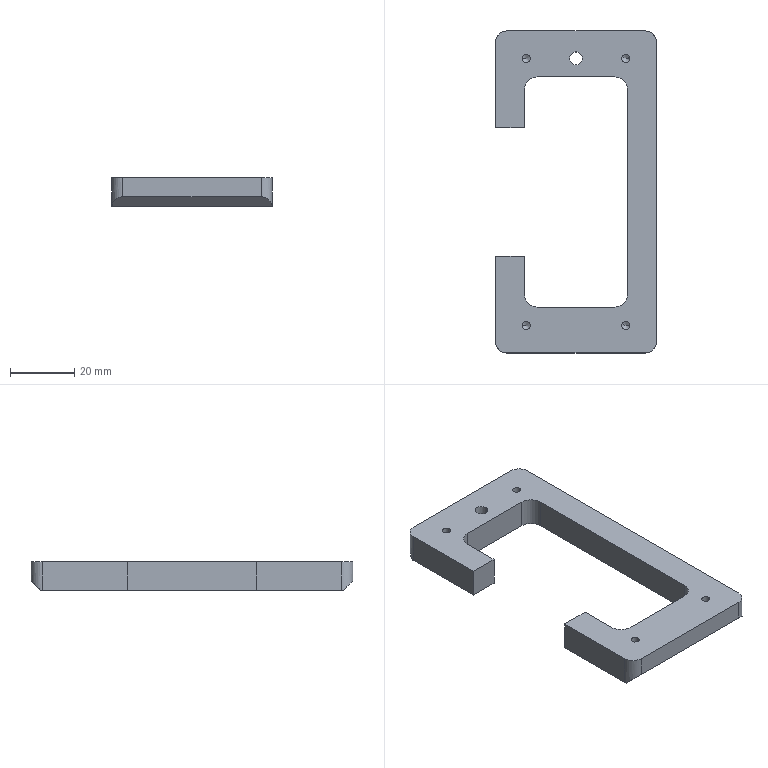Part | STEP file | X77-02213 | 1 solid | 42 faces | box 50 x 100 x 9 mm | volume 20503 mm3 | cylinder 18 | plane 16 | cone 8 | commonest cylinder face diameters 2.5 x8 7.116 x4 8 x4 4 x2
STEP:
#1=CARTESIAN_POINT('',(-2.,41.5,0.));
#2=VERTEX_POINT('',#1);
#3=CARTESIAN_POINT('',(2.,41.5,0.));
#4=VERTEX_POINT('',#3);
#5=CARTESIAN_POINT('',(-0.000000005,41.5,0.));
#6=DIRECTION('',(0.,0.,-1.));
#7=DIRECTION('',(1.,0.,0.));
#8=AXIS2_PLACEMENT_3D('',#5,#6,#7);
#9=CIRCLE('',#8,2.);
#10=EDGE_CURVE('',#2,#4,#9,.T.);
#11=ORIENTED_EDGE('',*,*,#10,.T.);
#12=CARTESIAN_POINT('',(2.,41.5,9.));
#13=VERTEX_POINT('',#12);
#14=CARTESIAN_POINT('',(2.,41.5,-1.));
#15=DIRECTION('',(0.,0.,1.));
#16=VECTOR('',#15,1000.);
#17=LINE('',#14,#16);
#18=EDGE_CURVE('',#4,#13,#17,.T.);
#19=ORIENTED_EDGE('',*,*,#18,.T.);
#20=CARTESIAN_POINT('',(-2.,41.5,9.));
#21=VERTEX_POINT('',#20);
#22=CARTESIAN_POINT('',(-0.000000005,41.5,9.));
#23=DIRECTION('',(0.,0.,1.));
#24=DIRECTION('',(-1.,0.,0.));
#25=AXIS2_PLACEMENT_3D('',#22,#23,#24);
#26=CIRCLE('',#25,2.);
#27=EDGE_CURVE('',#13,#21,#26,.T.);
#28=ORIENTED_EDGE('',*,*,#27,.T.);
#29=CARTESIAN_POINT('',(-2.,41.5,-1.));
#30=DIRECTION('',(0.,0.,1.));
#31=VECTOR('',#30,1000.);
#32=LINE('',#29,#31);
#33=EDGE_CURVE('',#2,#21,#32,.T.);
#34=ORIENTED_EDGE('',*,*,#33,.F.);
#35=EDGE_LOOP('',(#11,#19,#28,#34));
#36=FACE_OUTER_BOUND('',#35,.T.);
#37=CARTESIAN_POINT('',(-0.000000005,41.5,-1.));
#38=DIRECTION('',(0.,0.,1.));
#39=DIRECTION('',(-1.,0.,0.));
#40=AXIS2_PLACEMENT_3D('',#37,#38,#39);
#41=CYLINDRICAL_SURFACE('',#40,2.);
#42=ADVANCED_FACE('',(#36),#41,.F.);
#43=CARTESIAN_POINT('',(16.75,41.5,1.5));
#44=VERTEX_POINT('',#43);
#45=CARTESIAN_POINT('',(14.25,41.5,1.5));
#46=VERTEX_POINT('',#45);
#47=CARTESIAN_POINT('',(15.5,41.5,1.5));
#48=DIRECTION('',(0.,0.,1.));
#49=DIRECTION('',(-1.,0.,0.));
#50=AXIS2_PLACEMENT_3D('',#47,#48,#49);
#51=CIRCLE('',#50,1.25);
#52=EDGE_CURVE('',#44,#46,#51,.T.);
#53=ORIENTED_EDGE('',*,*,#52,.F.);
#54=CARTESIAN_POINT('',(16.75,41.5,9.));
#55=VERTEX_POINT('',#54);
#56=CARTESIAN_POINT('',(16.75,41.5,9.));
#57=DIRECTION('',(0.,0.,1.));
#58=VECTOR('',#57,1000.);
#59=LINE('',#56,#58);
#60=EDGE_CURVE('',#44,#55,#59,.T.);
#61=ORIENTED_EDGE('',*,*,#60,.T.);
#62=CARTESIAN_POINT('',(14.25,41.5,9.));
#63=VERTEX_POINT('',#62);
#64=CARTESIAN_POINT('',(15.5,41.5,9.));
#65=DIRECTION('',(0.,0.,1.));
#66=DIRECTION('',(-1.,0.,0.));
#67=AXIS2_PLACEMENT_3D('',#64,#65,#66);
#68=CIRCLE('',#67,1.25);
#69=EDGE_CURVE('',#55,#63,#68,.T.);
#70=ORIENTED_EDGE('',*,*,#69,.T.);
#71=CARTESIAN_POINT('',(14.25,41.5,9.));
#72=DIRECTION('',(0.,0.,1.));
#73=VECTOR('',#72,1000.);
#74=LINE('',#71,#73);
#75=EDGE_CURVE('',#46,#63,#74,.T.);
#76=ORIENTED_EDGE('',*,*,#75,.F.);
#77=EDGE_LOOP('',(#53,#61,#70,#76));
#78=FACE_OUTER_BOUND('',#77,.T.);
#79=CARTESIAN_POINT('',(15.5,41.5,9.));
#80=DIRECTION('',(0.,0.,1.));
#81=DIRECTION('',(-1.,0.,0.));
#82=AXIS2_PLACEMENT_3D('',#79,#80,#81);
#83=CYLINDRICAL_SURFACE('',#82,1.25);
#84=ADVANCED_FACE('',(#78),#83,.F.);
#85=CARTESIAN_POINT('',(15.5,41.5,0.7489));
#86=VERTEX_POINT('',#85);
#87=CARTESIAN_POINT('',(14.25,41.5,1.5));
#88=DIRECTION('',(-0.8572,0.,0.515));
#89=VECTOR('',#88,1000.);
#90=LINE('',#87,#89);
#91=EDGE_CURVE('',#86,#46,#90,.T.);
#92=ORIENTED_EDGE('',*,*,#91,.F.);
#93=CARTESIAN_POINT('',(16.75,41.5,1.5));
#94=DIRECTION('',(0.8572,0.,0.515));
#95=VECTOR('',#94,1000.);
#96=LINE('',#93,#95);
#97=EDGE_CURVE('',#86,#44,#96,.T.);
#98=ORIENTED_EDGE('',*,*,#97,.T.);
#99=ORIENTED_EDGE('',*,*,#52,.T.);
#100=EDGE_LOOP('',(#92,#98,#99));
#101=FACE_OUTER_BOUND('',#100,.T.);
#102=CARTESIAN_POINT('',(15.5,41.5,1.5));
#103=DIRECTION('',(0.,0.,1.));
#104=DIRECTION('',(-1.,0.,0.));
#105=AXIS2_PLACEMENT_3D('',#102,#103,#104);
#106=CONICAL_SURFACE('',#105,1.25,1.03);
#107=ADVANCED_FACE('',(#101),#106,.F.);
#108=CARTESIAN_POINT('',(-14.25,41.5,1.5));
#109=VERTEX_POINT('',#108);
#110=CARTESIAN_POINT('',(-16.75,41.5,1.5));
#111=VERTEX_POINT('',#110);
#112=CARTESIAN_POINT('',(-15.5,41.5,1.5));
#113=DIRECTION('',(0.,0.,1.));
#114=DIRECTION('',(-1.,0.,0.));
#115=AXIS2_PLACEMENT_3D('',#112,#113,#114);
#116=CIRCLE('',#115,1.25);
#117=EDGE_CURVE('',#109,#111,#116,.T.);
#118=ORIENTED_EDGE('',*,*,#117,.F.);
#119=CARTESIAN_POINT('',(-14.25,41.5,9.));
#120=VERTEX_POINT('',#119);
#121=CARTESIAN_POINT('',(-14.25,41.5,9.));
#122=DIRECTION('',(0.,0.,1.));
#123=VECTOR('',#122,1000.);
#124=LINE('',#121,#123);
#125=EDGE_CURVE('',#109,#120,#124,.T.);
#126=ORIENTED_EDGE('',*,*,#125,.T.);
#127=CARTESIAN_POINT('',(-16.75,41.5,9.));
#128=VERTEX_POINT('',#127);
#129=CARTESIAN_POINT('',(-15.5,41.5,9.));
#130=DIRECTION('',(0.,0.,1.));
#131=DIRECTION('',(-1.,0.,0.));
#132=AXIS2_PLACEMENT_3D('',#129,#130,#131);
#133=CIRCLE('',#132,1.25);
#134=EDGE_CURVE('',#120,#128,#133,.T.);
#135=ORIENTED_EDGE('',*,*,#134,.T.);
#136=CARTESIAN_POINT('',(-16.75,41.5,9.));
#137=DIRECTION('',(0.,0.,1.));
#138=VECTOR('',#137,1000.);
#139=LINE('',#136,#138);
#140=EDGE_CURVE('',#111,#128,#139,.T.);
#141=ORIENTED_EDGE('',*,*,#140,.F.);
#142=EDGE_LOOP('',(#118,#126,#135,#141));
#143=FACE_OUTER_BOUND('',#142,.T.);
#144=CARTESIAN_POINT('',(-15.5,41.5,9.));
#145=DIRECTION('',(0.,0.,1.));
#146=DIRECTION('',(-1.,0.,0.));
#147=AXIS2_PLACEMENT_3D('',#144,#145,#146);
#148=CYLINDRICAL_SURFACE('',#147,1.25);
#149=ADVANCED_FACE('',(#143),#148,.F.);
#150=CARTESIAN_POINT('',(-15.5,41.5,0.7489));
#151=VERTEX_POINT('',#150);
#152=CARTESIAN_POINT('',(-16.75,41.5,1.5));
#153=DIRECTION('',(-0.8572,0.,0.515));
#154=VECTOR('',#153,1000.);
#155=LINE('',#152,#154);
#156=EDGE_CURVE('',#151,#111,#155,.T.);
#157=ORIENTED_EDGE('',*,*,#156,.F.);
#158=CARTESIAN_POINT('',(-14.25,41.5,1.5));
#159=DIRECTION('',(0.8572,0.,0.515));
#160=VECTOR('',#159,1000.);
#161=LINE('',#158,#160);
#162=EDGE_CURVE('',#151,#109,#161,.T.);
#163=ORIENTED_EDGE('',*,*,#162,.T.);
#164=ORIENTED_EDGE('',*,*,#117,.T.);
#165=EDGE_LOOP('',(#157,#163,#164));
#166=FACE_OUTER_BOUND('',#165,.T.);
#167=CARTESIAN_POINT('',(-15.5,41.5,1.5));
#168=DIRECTION('',(0.,0.,1.));
#169=DIRECTION('',(-1.,0.,0.));
#170=AXIS2_PLACEMENT_3D('',#167,#168,#169);
#171=CONICAL_SURFACE('',#170,1.25,1.03);
#172=ADVANCED_FACE('',(#166),#171,.F.);
#173=CARTESIAN_POINT('',(-14.25,-41.5,1.5));
#174=VERTEX_POINT('',#173);
#175=CARTESIAN_POINT('',(-16.75,-41.5,1.5));
#176=VERTEX_POINT('',#175);
#177=CARTESIAN_POINT('',(-15.5,-41.5,1.5));
#178=DIRECTION('',(0.,0.,1.));
#179=DIRECTION('',(-1.,0.,0.));
#180=AXIS2_PLACEMENT_3D('',#177,#178,#179);
#181=CIRCLE('',#180,1.25);
#182=EDGE_CURVE('',#174,#176,#181,.T.);
#183=ORIENTED_EDGE('',*,*,#182,.F.);
#184=CARTESIAN_POINT('',(-14.25,-41.5,9.));
#185=VERTEX_POINT('',#184);
#186=CARTESIAN_POINT('',(-14.25,-41.5,9.));
#187=DIRECTION('',(0.,0.,1.));
#188=VECTOR('',#187,1000.);
#189=LINE('',#186,#188);
#190=EDGE_CURVE('',#174,#185,#189,.T.);
#191=ORIENTED_EDGE('',*,*,#190,.T.);
#192=CARTESIAN_POINT('',(-16.75,-41.5,9.));
#193=VERTEX_POINT('',#192);
#194=CARTESIAN_POINT('',(-15.5,-41.5,9.));
#195=DIRECTION('',(0.,0.,1.));
#196=DIRECTION('',(-1.,0.,0.));
#197=AXIS2_PLACEMENT_3D('',#194,#195,#196);
#198=CIRCLE('',#197,1.25);
#199=EDGE_CURVE('',#185,#193,#198,.T.);
#200=ORIENTED_EDGE('',*,*,#199,.T.);
#201=CARTESIAN_POINT('',(-16.75,-41.5,9.));
#202=DIRECTION('',(0.,0.,1.));
#203=VECTOR('',#202,1000.);
#204=LINE('',#201,#203);
#205=EDGE_CURVE('',#176,#193,#204,.T.);
#206=ORIENTED_EDGE('',*,*,#205,.F.);
#207=EDGE_LOOP('',(#183,#191,#200,#206));
#208=FACE_OUTER_BOUND('',#207,.T.);
#209=CARTESIAN_POINT('',(-15.5,-41.5,9.));
#210=DIRECTION('',(0.,0.,1.));
#211=DIRECTION('',(-1.,0.,0.));
#212=AXIS2_PLACEMENT_3D('',#209,#210,#211);
#213=CYLINDRICAL_SURFACE('',#212,1.25);
#214=ADVANCED_FACE('',(#208),#213,.F.);
#215=CARTESIAN_POINT('',(-15.5,-41.5,0.7489));
#216=VERTEX_POINT('',#215);
#217=CARTESIAN_POINT('',(-16.75,-41.5,1.5));
#218=DIRECTION('',(-0.8572,0.,0.515));
#219=VECTOR('',#218,1000.);
#220=LINE('',#217,#219);
#221=EDGE_CURVE('',#216,#176,#220,.T.);
#222=ORIENTED_EDGE('',*,*,#221,.F.);
#223=CARTESIAN_POINT('',(-14.25,-41.5,1.5));
#224=DIRECTION('',(0.8572,0.,0.515));
#225=VECTOR('',#224,1000.);
#226=LINE('',#223,#225);
#227=EDGE_CURVE('',#216,#174,#226,.T.);
#228=ORIENTED_EDGE('',*,*,#227,.T.);
#229=ORIENTED_EDGE('',*,*,#182,.T.);
#230=EDGE_LOOP('',(#222,#228,#229));
#231=FACE_OUTER_BOUND('',#230,.T.);
#232=CARTESIAN_POINT('',(-15.5,-41.5,1.5));
#233=DIRECTION('',(0.,0.,1.));
#234=DIRECTION('',(-1.,0.,0.));
#235=AXIS2_PLACEMENT_3D('',#232,#233,#234);
#236=CONICAL_SURFACE('',#235,1.25,1.03);
#237=ADVANCED_FACE('',(#231),#236,.F.);
#238=CARTESIAN_POINT('',(16.75,-41.5,1.5));
#239=VERTEX_POINT('',#238);
#240=CARTESIAN_POINT('',(14.25,-41.5,1.5));
#241=VERTEX_POINT('',#240);
#242=CARTESIAN_POINT('',(15.5,-41.5,1.5));
#243=DIRECTION('',(0.,0.,1.));
#244=DIRECTION('',(-1.,0.,0.));
#245=AXIS2_PLACEMENT_3D('',#242,#243,#244);
#246=CIRCLE('',#245,1.25);
#247=EDGE_CURVE('',#239,#241,#246,.T.);
#248=ORIENTED_EDGE('',*,*,#247,.F.);
#249=CARTESIAN_POINT('',(16.75,-41.5,9.));
#250=VERTEX_POINT('',#249);
#251=CARTESIAN_POINT('',(16.75,-41.5,9.));
#252=DIRECTION('',(0.,0.,1.));
#253=VECTOR('',#252,1000.);
#254=LINE('',#251,#253);
#255=EDGE_CURVE('',#239,#250,#254,.T.);
#256=ORIENTED_EDGE('',*,*,#255,.T.);
#257=CARTESIAN_POINT('',(14.25,-41.5,9.));
#258=VERTEX_POINT('',#257);
#259=CARTESIAN_POINT('',(15.5,-41.5,9.));
#260=DIRECTION('',(0.,0.,1.));
#261=DIRECTION('',(-1.,0.,0.));
#262=AXIS2_PLACEMENT_3D('',#259,#260,#261);
#263=CIRCLE('',#262,1.25);
#264=EDGE_CURVE('',#250,#258,#263,.T.);
#265=ORIENTED_EDGE('',*,*,#264,.T.);
#266=CARTESIAN_POINT('',(14.25,-41.5,9.));
#267=DIRECTION('',(0.,0.,1.));
#268=VECTOR('',#267,1000.);
#269=LINE('',#266,#268);
#270=EDGE_CURVE('',#241,#258,#269,.T.);
#271=ORIENTED_EDGE('',*,*,#270,.F.);
#272=EDGE_LOOP('',(#248,#256,#265,#271));
#273=FACE_OUTER_BOUND('',#272,.T.);
#274=CARTESIAN_POINT('',(15.5,-41.5,9.));
#275=DIRECTION('',(0.,0.,1.));
#276=DIRECTION('',(-1.,0.,0.));
#277=AXIS2_PLACEMENT_3D('',#274,#275,#276);
#278=CYLINDRICAL_SURFACE('',#277,1.25);
#279=ADVANCED_FACE('',(#273),#278,.F.);
#280=CARTESIAN_POINT('',(15.5,-41.5,0.7489));
#281=VERTEX_POINT('',#280);
#282=CARTESIAN_POINT('',(14.25,-41.5,1.5));
#283=DIRECTION('',(-0.8572,0.,0.515));
#284=VECTOR('',#283,1000.);
#285=LINE('',#282,#284);
#286=EDGE_CURVE('',#281,#241,#285,.T.);
#287=ORIENTED_EDGE('',*,*,#286,.F.);
#288=CARTESIAN_POINT('',(16.75,-41.5,1.5));
#289=DIRECTION('',(0.8572,0.,0.515));
#290=VECTOR('',#289,1000.);
#291=LINE('',#288,#290);
#292=EDGE_CURVE('',#281,#239,#291,.T.);
#293=ORIENTED_EDGE('',*,*,#292,.T.);
#294=ORIENTED_EDGE('',*,*,#247,.T.);
#295=EDGE_LOOP('',(#287,#293,#294));
#296=FACE_OUTER_BOUND('',#295,.T.);
#297=CARTESIAN_POINT('',(15.5,-41.5,1.5));
#298=DIRECTION('',(0.,0.,1.));
#299=DIRECTION('',(-1.,0.,0.));
#300=AXIS2_PLACEMENT_3D('',#297,#298,#299);
#301=CONICAL_SURFACE('',#300,1.25,1.03);
#302=ADVANCED_FACE('',(#296),#301,.F.);
#303=CARTESIAN_POINT('',(-25.,-20.,9.));
#304=VERTEX_POINT('',#303);
#305=CARTESIAN_POINT('',(-25.,-46.442,9.));
#306=VERTEX_POINT('',#305);
#307=CARTESIAN_POINT('',(-25.,50.,9.));
#308=DIRECTION('',(0.,-1.,0.));
#309=VECTOR('',#308,1000.);
#310=LINE('',#307,#309);
#311=EDGE_CURVE('',#304,#306,#310,.T.);
#312=ORIENTED_EDGE('',*,*,#311,.F.);
#313=CARTESIAN_POINT('',(-25.,-20.,0.));
#314=VERTEX_POINT('',#313);
#315=CARTESIAN_POINT('',(-25.,-20.,-11.867));
#316=DIRECTION('',(0.,0.,1.));
#317=VECTOR('',#316,1000.);
#318=LINE('',#315,#317);
#319=EDGE_CURVE('',#314,#304,#318,.T.);
#320=ORIENTED_EDGE('',*,*,#319,.F.);
#321=CARTESIAN_POINT('',(-25.,-46.442,0.));
#322=VERTEX_POINT('',#321);
#323=CARTESIAN_POINT('',(-25.,46.442,0.));
#324=DIRECTION('',(0.,-1.,0.));
#325=VECTOR('',#324,1000.);
#326=LINE('',#323,#325);
#327=EDGE_CURVE('',#314,#322,#326,.T.);
#328=ORIENTED_EDGE('',*,*,#327,.T.);
#329=CARTESIAN_POINT('',(-25.,-46.442,10.));
#330=DIRECTION('',(0.,0.,-1.));
#331=VECTOR('',#330,1000.);
#332=LINE('',#329,#331);
#333=EDGE_CURVE('',#306,#322,#332,.T.);
#334=ORIENTED_EDGE('',*,*,#333,.F.);
#335=EDGE_LOOP('',(#312,#320,#328,#334));
#336=FACE_OUTER_BOUND('',#335,.T.);
#337=CARTESIAN_POINT('',(-25.,46.442,10.));
#338=DIRECTION('',(1.,0.,0.));
#339=DIRECTION('',(0.,0.,-1.));
#340=AXIS2_PLACEMENT_3D('',#337,#338,#339);
#341=PLANE('',#340);
#342=ADVANCED_FACE('',(#336),#341,.F.);
#343=CARTESIAN_POINT('',(-16.,-20.,9.));
#344=VERTEX_POINT('',#343);
#345=CARTESIAN_POINT('',(-16.,-20.,0.));
#346=VERTEX_POINT('',#345);
#347=CARTESIAN_POINT('',(-16.,-20.,10.));
#348=DIRECTION('',(0.,0.,-1.));
#349=VECTOR('',#348,1000.);
#350=LINE('',#347,#349);
#351=EDGE_CURVE('',#344,#346,#350,.T.);
#352=ORIENTED_EDGE('',*,*,#351,.F.);
#353=CARTESIAN_POINT('',(-16.,-31.75,9.));
#354=VERTEX_POINT('',#353);
#355=CARTESIAN_POINT('',(-16.,-31.75,9.));
#356=DIRECTION('',(0.,1.,0.));
#357=VECTOR('',#356,1000.);
#358=LINE('',#355,#357);
#359=EDGE_CURVE('',#354,#344,#358,.T.);
#360=ORIENTED_EDGE('',*,*,#359,.F.);
#361=CARTESIAN_POINT('',(-16.,-31.75,0.));
#362=VERTEX_POINT('',#361);
#363=CARTESIAN_POINT('',(-16.,-31.75,10.));
#364=DIRECTION('',(0.,0.,-1.));
#365=VECTOR('',#364,1000.);
#366=LINE('',#363,#365);
#367=EDGE_CURVE('',#354,#362,#366,.T.);
#368=ORIENTED_EDGE('',*,*,#367,.T.);
#369=CARTESIAN_POINT('',(-16.,-31.75,0.));
#370=DIRECTION('',(0.,-1.,0.));
#371=VECTOR('',#370,1000.);
#372=LINE('',#369,#371);
#373=EDGE_CURVE('',#346,#362,#372,.T.);
#374=ORIENTED_EDGE('',*,*,#373,.F.);
#375=EDGE_LOOP('',(#352,#360,#368,#374));
#376=FACE_OUTER_BOUND('',#375,.T.);
#377=CARTESIAN_POINT('',(-16.,-31.75,10.));
#378=DIRECTION('',(1.,0.,0.));
#379=DIRECTION('',(0.,1.,0.));
#380=AXIS2_PLACEMENT_3D('',#377,#378,#379);
#381=PLANE('',#380);
#382=ADVANCED_FACE('',(#376),#381,.T.);
#383=CARTESIAN_POINT('',(21.442,-20.,0.));
#384=DIRECTION('',(-1.,0.,0.));
#385=VECTOR('',#384,1000.);
#386=LINE('',#383,#385);
#387=EDGE_CURVE('',#346,#314,#386,.T.);
#388=ORIENTED_EDGE('',*,*,#387,.F.);
#389=ORIENTED_EDGE('',*,*,#373,.T.);
#390=CARTESIAN_POINT('',(-12.,-35.75,0.));
#391=VERTEX_POINT('',#390);
#392=CARTESIAN_POINT('',(-12.,-31.75,0.));
#393=DIRECTION('',(0.,0.,1.));
#394=DIRECTION('',(-1.,0.,0.));
#395=AXIS2_PLACEMENT_3D('',#392,#393,#394);
#396=CIRCLE('',#395,4.);
#397=EDGE_CURVE('',#362,#391,#396,.T.);
#398=ORIENTED_EDGE('',*,*,#397,.T.);
#399=CARTESIAN_POINT('',(12.,-35.75,0.));
#400=VERTEX_POINT('',#399);
#401=CARTESIAN_POINT('',(-12.,-35.75,0.));
#402=DIRECTION('',(1.,0.,0.));
#403=VECTOR('',#402,1000.);
#404=LINE('',#401,#403);
#405=EDGE_CURVE('',#391,#400,#404,.T.);
#406=ORIENTED_EDGE('',*,*,#405,.T.);
#407=CARTESIAN_POINT('',(16.,-31.75,0.));
#408=VERTEX_POINT('',#407);
#409=CARTESIAN_POINT('',(12.,-31.75,0.));
#410=DIRECTION('',(0.,0.,1.));
#411=DIRECTION('',(-1.,0.,0.));
#412=AXIS2_PLACEMENT_3D('',#409,#410,#411);
#413=CIRCLE('',#412,4.);
#414=EDGE_CURVE('',#400,#408,#413,.T.);
#415=ORIENTED_EDGE('',*,*,#414,.T.);
#416=CARTESIAN_POINT('',(16.,31.75,0.));
#417=VERTEX_POINT('',#416);
#418=CARTESIAN_POINT('',(16.,-31.75,0.));
#419=DIRECTION('',(0.,1.,0.));
#420=VECTOR('',#419,1000.);
#421=LINE('',#418,#420);
#422=EDGE_CURVE('',#408,#417,#421,.T.);
#423=ORIENTED_EDGE('',*,*,#422,.T.);
#424=CARTESIAN_POINT('',(12.,35.75,0.));
#425=VERTEX_POINT('',#424);
#426=CARTESIAN_POINT('',(12.,31.75,0.));
#427=DIRECTION('',(0.,0.,1.));
#428=DIRECTION('',(1.,0.,0.));
#429=AXIS2_PLACEMENT_3D('',#426,#427,#428);
#430=CIRCLE('',#429,4.);
#431=EDGE_CURVE('',#417,#425,#430,.T.);
#432=ORIENTED_EDGE('',*,*,#431,.T.);
#433=CARTESIAN_POINT('',(-12.,35.75,0.));
#434=VERTEX_POINT('',#433);
#435=CARTESIAN_POINT('',(-12.,35.75,0.));
#436=DIRECTION('',(-1.,0.,0.));
#437=VECTOR('',#436,1000.);
#438=LINE('',#435,#437);
#439=EDGE_CURVE('',#425,#434,#438,.T.);
#440=ORIENTED_EDGE('',*,*,#439,.T.);
#441=CARTESIAN_POINT('',(-16.,31.75,0.));
#442=VERTEX_POINT('',#441);
#443=CARTESIAN_POINT('',(-12.,31.75,0.));
#444=DIRECTION('',(0.,0.,1.));
#445=DIRECTION('',(1.,0.,0.));
#446=AXIS2_PLACEMENT_3D('',#443,#444,#445);
#447=CIRCLE('',#446,4.);
#448=EDGE_CURVE('',#434,#442,#447,.T.);
#449=ORIENTED_EDGE('',*,*,#448,.T.);
#450=CARTESIAN_POINT('',(-16.,20.,0.));
#451=VERTEX_POINT('',#450);
#452=CARTESIAN_POINT('',(-16.,-31.75,0.));
#453=DIRECTION('',(0.,-1.,0.));
#454=VECTOR('',#453,1000.);
#455=LINE('',#452,#454);
#456=EDGE_CURVE('',#442,#451,#455,.T.);
#457=ORIENTED_EDGE('',*,*,#456,.T.);
#458=CARTESIAN_POINT('',(-25.,20.,0.));
#459=VERTEX_POINT('',#458);
#460=CARTESIAN_POINT('',(21.442,20.,0.));
#461=DIRECTION('',(1.,0.,0.));
#462=VECTOR('',#461,1000.);
#463=LINE('',#460,#462);
#464=EDGE_CURVE('',#459,#451,#463,.T.);
#465=ORIENTED_EDGE('',*,*,#464,.F.);
#466=CARTESIAN_POINT('',(-25.,46.442,0.));
#467=VERTEX_POINT('',#466);
#468=CARTESIAN_POINT('',(-25.,46.442,0.));
#469=DIRECTION('',(0.,-1.,0.));
#470=VECTOR('',#469,1000.);
#471=LINE('',#468,#470);
#472=EDGE_CURVE('',#467,#459,#471,.T.);
#473=ORIENTED_EDGE('',*,*,#472,.F.);
#474=CARTESIAN_POINT('',(-24.956,47.,0.));
#475=VERTEX_POINT('',#474);
#476=CARTESIAN_POINT('',(-21.442,46.442,0.));
#477=DIRECTION('',(0.,0.,1.));
#478=DIRECTION('',(1.,0.,0.));
#479=AXIS2_PLACEMENT_3D('',#476,#477,#478);
#480=CIRCLE('',#479,3.558);
#481=EDGE_CURVE('',#475,#467,#480,.T.);
#482=ORIENTED_EDGE('',*,*,#481,.F.);
#483=CARTESIAN_POINT('',(24.956,47.,0.));
#484=VERTEX_POINT('',#483);
#485=CARTESIAN_POINT('',(-25.,47.,0.));
#486=DIRECTION('',(1.,0.,0.));
#487=VECTOR('',#486,1000.);
#488=LINE('',#485,#487);
#489=EDGE_CURVE('',#475,#484,#488,.T.);
#490=ORIENTED_EDGE('',*,*,#489,.T.);
#491=CARTESIAN_POINT('',(25.,46.442,0.));
#492=VERTEX_POINT('',#491);
#493=CARTESIAN_POINT('',(21.442,46.442,0.));
#494=DIRECTION('',(0.,0.,1.));
#495=DIRECTION('',(-1.,0.,0.));
#496=AXIS2_PLACEMENT_3D('',#493,#494,#495);
#497=CIRCLE('',#496,3.558);
#498=EDGE_CURVE('',#492,#484,#497,.T.);
#499=ORIENTED_EDGE('',*,*,#498,.F.);
#500=CARTESIAN_POINT('',(25.,-46.442,0.));
#501=VERTEX_POINT('',#500);
#502=CARTESIAN_POINT('',(25.,46.442,0.));
#503=DIRECTION('',(0.,1.,0.));
#504=VECTOR('',#503,1000.);
#505=LINE('',#502,#504);
#506=EDGE_CURVE('',#501,#492,#505,.T.);
#507=ORIENTED_EDGE('',*,*,#506,.F.);
#508=CARTESIAN_POINT('',(24.956,-47.,0.));
#509=VERTEX_POINT('',#508);
#510=CARTESIAN_POINT('',(21.442,-46.442,0.));
#511=DIRECTION('',(0.,0.,1.));
#512=DIRECTION('',(1.,0.,0.));
#513=AXIS2_PLACEMENT_3D('',#510,#511,#512);
#514=CIRCLE('',#513,3.558);
#515=EDGE_CURVE('',#509,#501,#514,.T.);
#516=ORIENTED_EDGE('',*,*,#515,.F.);
#517=CARTESIAN_POINT('',(-24.956,-47.,0.));
#518=VERTEX_POINT('',#517);
#519=CARTESIAN_POINT('',(-25.,-47.,0.));
#520=DIRECTION('',(1.,0.,0.));
#521=VECTOR('',#520,1000.);
#522=LINE('',#519,#521);
#523=EDGE_CURVE('',#518,#509,#522,.T.);
#524=ORIENTED_EDGE('',*,*,#523,.F.);
#525=CARTESIAN_POINT('',(-21.442,-46.442,0.));
#526=DIRECTION('',(0.,0.,1.));
#527=DIRECTION('',(1.,0.,0.));
#528=AXIS2_PLACEMENT_3D('',#525,#526,#527);
#529=CIRCLE('',#528,3.558);
#530=EDGE_CURVE('',#322,#518,#529,.T.);
#531=ORIENTED_EDGE('',*,*,#530,.F.);
#532=ORIENTED_EDGE('',*,*,#327,.F.);
#533=EDGE_LOOP('',(#388,#389,#398,#406,#415,#423,#432,#440,#449,#457,#465,#473,#482,#490,#499,#507,#516,#524,#531,#532));
#534=FACE_OUTER_BOUND('',#533,.T.);
#535=ORIENTED_EDGE('',*,*,#10,.F.);
#536=CARTESIAN_POINT('',(-0.000000005,41.5,0.));
#537=DIRECTION('',(0.,0.,-1.));
#538=DIRECTION('',(1.,0.,0.));
#539=AXIS2_PLACEMENT_3D('',#536,#537,#538);
#540=CIRCLE('',#539,2.);
#541=EDGE_CURVE('',#4,#2,#540,.T.);
#542=ORIENTED_EDGE('',*,*,#541,.F.);
#543=EDGE_LOOP('',(#535,#542));
#544=FACE_BOUND('',#543,.T.);
#545=CARTESIAN_POINT('',(21.442,46.442,0.));
#546=DIRECTION('',(0.,0.,-1.));
#547=DIRECTION('',(-1.,0.,0.));
#548=AXIS2_PLACEMENT_3D('',#545,#546,#547);
#549=PLANE('',#548);
#550=ADVANCED_FACE('',(#534,#544),#549,.T.);
#551=CARTESIAN_POINT('',(21.442,50.,9.));
#552=VERTEX_POINT('',#551);
#553=CARTESIAN_POINT('',(21.442,50.,3.));
#554=VERTEX_POINT('',#553);
#555=CARTESIAN_POINT('',(21.442,50.,10.));
#556=DIRECTION('',(0.,0.,-1.));
#557=VECTOR('',#556,1000.);
#558=LINE('',#555,#557);
#559=EDGE_CURVE('',#552,#554,#558,.T.);
#560=ORIENTED_EDGE('',*,*,#559,.F.);
#561=CARTESIAN_POINT('',(25.,46.442,9.));
#562=VERTEX_POINT('',#561);
#563=CARTESIAN_POINT('',(21.442,46.442,9.));
#564=DIRECTION('',(0.,0.,-1.));
#565=DIRECTION('',(1.,0.,0.));
#566=AXIS2_PLACEMENT_3D('',#563,#564,#565);
#567=CIRCLE('',#566,3.558);
#568=EDGE_CURVE('',#552,#562,#567,.T.);
#569=ORIENTED_EDGE('',*,*,#568,.T.);
#570=CARTESIAN_POINT('',(25.,46.442,10.));
#571=DIRECTION('',(0.,0.,-1.));
#572=VECTOR('',#571,1000.);
#573=LINE('',#570,#572);
#574=EDGE_CURVE('',#562,#492,#573,.T.);
#575=ORIENTED_EDGE('',*,*,#574,.T.);
#576=ORIENTED_EDGE('',*,*,#498,.T.);
#577=CARTESIAN_POINT('',(24.956,47.,0.));
#578=CARTESIAN_POINT('',(24.669,48.81,1.81));
#579=CARTESIAN_POINT('',(23.275,50.,3.));
#580=CARTESIAN_POINT('',(21.442,50.,3.));
#581=(BOUNDED_CURVE()B_SPLINE_CURVE(3,(#577,#578,#579,#580),.UNSPECIFIED.,.F.,.F.)B_SPLINE_CURVE_WITH_KNOTS((4,4),(1.728,3.142),.UNSPECIFIED.)CURVE()GEOMETRIC_REPRESENTATION_ITEM()RATIONAL_B_SPLINE_CURVE((1.,0.8404,0.8404,1.))REPRESENTATION_ITEM(''));
#582=EDGE_CURVE('',#484,#554,#581,.T.);
#583=ORIENTED_EDGE('',*,*,#582,.T.);
#584=EDGE_LOOP('',(#560,#569,#575,#576,#583));
#585=FACE_OUTER_BOUND('',#584,.T.);
#586=CARTESIAN_POINT('',(21.442,46.442,10.));
#587=DIRECTION('',(0.,0.,-1.));
#588=DIRECTION('',(-1.,0.,0.));
#589=AXIS2_PLACEMENT_3D('',#586,#587,#588);
#590=CYLINDRICAL_SURFACE('',#589,3.558);
#591=ADVANCED_FACE('',(#585),#590,.T.);
#592=CARTESIAN_POINT('',(-21.442,50.,9.));
#593=VERTEX_POINT('',#592);
#594=CARTESIAN_POINT('',(-21.442,50.,3.));
#595=VERTEX_POINT('',#594);
#596=CARTESIAN_POINT('',(-21.442,50.,10.));
#597=DIRECTION('',(0.,0.,-1.));
#598=VECTOR('',#597,1000.);
#599=LINE('',#596,#598);
#600=EDGE_CURVE('',#593,#595,#599,.T.);
#601=ORIENTED_EDGE('',*,*,#600,.F.);
#602=CARTESIAN_POINT('',(25.,50.,9.));
#603=DIRECTION('',(1.,0.,0.));
#604=VECTOR('',#603,1000.);
#605=LINE('',#602,#604);
#606=EDGE_CURVE('',#593,#552,#605,.T.);
#607=ORIENTED_EDGE('',*,*,#606,.T.);
#608=ORIENTED_EDGE('',*,*,#559,.T.);
#609=CARTESIAN_POINT('',(-25.,50.,3.));
#610=DIRECTION('',(1.,0.,0.));
#611=VECTOR('',#610,1000.);
#612=LINE('',#609,#611);
#613=EDGE_CURVE('',#595,#554,#612,.T.);
#614=ORIENTED_EDGE('',*,*,#613,.F.);
#615=EDGE_LOOP('',(#601,#607,#608,#614));
#616=FACE_OUTER_BOUND('',#615,.T.);
#617=CARTESIAN_POINT('',(-21.442,50.,10.));
#618=DIRECTION('',(0.,-1.,0.));
#619=DIRECTION('',(0.,0.,-1.));
#620=AXIS2_PLACEMENT_3D('',#617,#618,#619);
#621=PLANE('',#620);
#622=ADVANCED_FACE('',(#616),#621,.F.);
#623=CARTESIAN_POINT('',(-25.,46.442,9.));
#624=VERTEX_POINT('',#623);
#625=CARTESIAN_POINT('',(-25.,46.442,10.));
#626=DIRECTION('',(0.,0.,-1.));
#627=VECTOR('',#626,1000.);
#628=LINE('',#625,#627);
#629=EDGE_CURVE('',#624,#467,#628,.T.);
#630=ORIENTED_EDGE('',*,*,#629,.F.);
#631=CARTESIAN_POINT('',(-21.442,46.442,9.));
#632=DIRECTION('',(0.,0.,-1.));
#633=DIRECTION('',(1.,0.,0.));
#634=AXIS2_PLACEMENT_3D('',#631,#632,#633);
#635=CIRCLE('',#634,3.558);
#636=EDGE_CURVE('',#624,#593,#635,.T.);
#637=ORIENTED_EDGE('',*,*,#636,.T.);
#638=ORIENTED_EDGE('',*,*,#600,.T.);
#639=CARTESIAN_POINT('',(-21.442,50.,3.));
#640=CARTESIAN_POINT('',(-23.275,50.,3.));
#641=CARTESIAN_POINT('',(-24.669,48.81,1.81));
#642=CARTESIAN_POINT('',(-24.956,47.,0.));
#643=(BOUNDED_CURVE()B_SPLINE_CURVE(3,(#639,#640,#641,#642),.UNSPECIFIED.,.F.,.T.)B_SPLINE_CURVE_WITH_KNOTS((4,4),(3.142,4.555),.UNSPECIFIED.)CURVE()GEOMETRIC_REPRESENTATION_ITEM()RATIONAL_B_SPLINE_CURVE((1.,0.8404,0.8404,1.))REPRESENTATION_ITEM(''));
#644=EDGE_CURVE('',#595,#475,#643,.T.);
#645=ORIENTED_EDGE('',*,*,#644,.T.);
#646=ORIENTED_EDGE('',*,*,#481,.T.);
#647=EDGE_LOOP('',(#630,#637,#638,#645,#646));
#648=FACE_OUTER_BOUND('',#647,.T.);
#649=CARTESIAN_POINT('',(-21.442,46.442,10.));
#650=DIRECTION('',(0.,0.,-1.));
#651=DIRECTION('',(-1.,0.,0.));
#652=AXIS2_PLACEMENT_3D('',#649,#650,#651);
#653=CYLINDRICAL_SURFACE('',#652,3.558);
#654=ADVANCED_FACE('',(#648),#653,.T.);
#655=ORIENTED_EDGE('',*,*,#472,.T.);
#656=CARTESIAN_POINT('',(-25.,20.,9.));
#657=VERTEX_POINT('',#656);
#658=CARTESIAN_POINT('',(-25.,20.,-11.867));
#659=DIRECTION('',(0.,0.,-1.));
#660=VECTOR('',#659,1000.);
#661=LINE('',#658,#660);
#662=EDGE_CURVE('',#657,#459,#661,.T.);
#663=ORIENTED_EDGE('',*,*,#662,.F.);
#664=CARTESIAN_POINT('',(-25.,50.,9.));
#665=DIRECTION('',(0.,-1.,0.));
#666=VECTOR('',#665,1000.);
#667=LINE('',#664,#666);
#668=EDGE_CURVE('',#624,#657,#667,.T.);
#669=ORIENTED_EDGE('',*,*,#668,.F.);
#670=ORIENTED_EDGE('',*,*,#629,.T.);
#671=EDGE_LOOP('',(#655,#663,#669,#670));
#672=FACE_OUTER_BOUND('',#671,.T.);
#673=CARTESIAN_POINT('',(-25.,46.442,10.));
#674=DIRECTION('',(1.,0.,0.));
#675=DIRECTION('',(0.,0.,-1.));
#676=AXIS2_PLACEMENT_3D('',#673,#674,#675);
#677=PLANE('',#676);
#678=ADVANCED_FACE('',(#672),#677,.F.);
#679=CARTESIAN_POINT('',(-21.442,-50.,9.));
#680=VERTEX_POINT('',#679);
#681=CARTESIAN_POINT('',(-21.442,-50.,3.));
#682=VERTEX_POINT('',#681);
#683=CARTESIAN_POINT('',(-21.442,-50.,10.));
#684=DIRECTION('',(0.,0.,-1.));
#685=VECTOR('',#684,1000.);
#686=LINE('',#683,#685);
#687=EDGE_CURVE('',#680,#682,#686,.T.);
#688=ORIENTED_EDGE('',*,*,#687,.F.);
#689=CARTESIAN_POINT('',(-21.442,-46.442,9.));
#690=DIRECTION('',(0.,0.,-1.));
#691=DIRECTION('',(1.,0.,0.));
#692=AXIS2_PLACEMENT_3D('',#689,#690,#691);
#693=CIRCLE('',#692,3.558);
#694=EDGE_CURVE('',#680,#306,#693,.T.);
#695=ORIENTED_EDGE('',*,*,#694,.T.);
#696=ORIENTED_EDGE('',*,*,#333,.T.);
#697=ORIENTED_EDGE('',*,*,#530,.T.);
#698=CARTESIAN_POINT('',(-24.956,-47.,0.));
#699=CARTESIAN_POINT('',(-24.669,-48.81,1.81));
#700=CARTESIAN_POINT('',(-23.275,-50.,3.));
#701=CARTESIAN_POINT('',(-21.442,-50.,3.));
#702=(BOUNDED_CURVE()B_SPLINE_CURVE(3,(#698,#699,#700,#701),.UNSPECIFIED.,.F.,.F.)B_SPLINE_CURVE_WITH_KNOTS((4,4),(1.728,3.142),.UNSPECIFIED.)CURVE()GEOMETRIC_REPRESENTATION_ITEM()RATIONAL_B_SPLINE_CURVE((1.,0.8404,0.8404,1.))REPRESENTATION_ITEM(''));
#703=EDGE_CURVE('',#518,#682,#702,.T.);
#704=ORIENTED_EDGE('',*,*,#703,.T.);
#705=EDGE_LOOP('',(#688,#695,#696,#697,#704));
#706=FACE_OUTER_BOUND('',#705,.T.);
#707=CARTESIAN_POINT('',(-21.442,-46.442,10.));
#708=DIRECTION('',(0.,0.,-1.));
#709=DIRECTION('',(-1.,0.,0.));
#710=AXIS2_PLACEMENT_3D('',#707,#708,#709);
#711=CYLINDRICAL_SURFACE('',#710,3.558);
#712=ADVANCED_FACE('',(#706),#711,.T.);
#713=CARTESIAN_POINT('',(21.442,-50.,9.));
#714=VERTEX_POINT('',#713);
#715=CARTESIAN_POINT('',(21.442,-50.,3.));
#716=VERTEX_POINT('',#715);
#717=CARTESIAN_POINT('',(21.442,-50.,10.));
#718=DIRECTION('',(0.,0.,-1.));
#719=VECTOR('',#718,1000.);
#720=LINE('',#717,#719);
#721=EDGE_CURVE('',#714,#716,#720,.T.);
#722=ORIENTED_EDGE('',*,*,#721,.F.);
#723=CARTESIAN_POINT('',(25.,-50.,9.));
#724=DIRECTION('',(1.,0.,0.));
#725=VECTOR('',#724,1000.);
#726=LINE('',#723,#725);
#727=EDGE_CURVE('',#680,#714,#726,.T.);
#728=ORIENTED_EDGE('',*,*,#727,.F.);
#729=ORIENTED_EDGE('',*,*,#687,.T.);
#730=CARTESIAN_POINT('',(-25.,-50.,3.));
#731=DIRECTION('',(1.,0.,0.));
#732=VECTOR('',#731,1000.);
#733=LINE('',#730,#732);
#734=EDGE_CURVE('',#682,#716,#733,.T.);
#735=ORIENTED_EDGE('',*,*,#734,.T.);
#736=EDGE_LOOP('',(#722,#728,#729,#735));
#737=FACE_OUTER_BOUND('',#736,.T.);
#738=CARTESIAN_POINT('',(-21.442,-50.,10.));
#739=DIRECTION('',(0.,1.,0.));
#740=DIRECTION('',(0.,0.,1.));
#741=AXIS2_PLACEMENT_3D('',#738,#739,#740);
#742=PLANE('',#741);
#743=ADVANCED_FACE('',(#737),#742,.F.);
#744=CARTESIAN_POINT('',(25.,-46.442,9.));
#745=VERTEX_POINT('',#744);
#746=CARTESIAN_POINT('',(25.,-46.442,10.));
#747=DIRECTION('',(0.,0.,-1.));
#748=VECTOR('',#747,1000.);
#749=LINE('',#746,#748);
#750=EDGE_CURVE('',#745,#501,#749,.T.);
#751=ORIENTED_EDGE('',*,*,#750,.F.);
#752=CARTESIAN_POINT('',(21.442,-46.442,9.));
#753=DIRECTION('',(0.,0.,-1.));
#754=DIRECTION('',(1.,0.,0.));
#755=AXIS2_PLACEMENT_3D('',#752,#753,#754);
#756=CIRCLE('',#755,3.558);
#757=EDGE_CURVE('',#745,#714,#756,.T.);
#758=ORIENTED_EDGE('',*,*,#757,.T.);
#759=ORIENTED_EDGE('',*,*,#721,.T.);
#760=CARTESIAN_POINT('',(21.442,-50.,3.));
#761=CARTESIAN_POINT('',(23.275,-50.,3.));
#762=CARTESIAN_POINT('',(24.669,-48.81,1.81));
#763=CARTESIAN_POINT('',(24.956,-47.,0.));
#764=(BOUNDED_CURVE()B_SPLINE_CURVE(3,(#760,#761,#762,#763),.UNSPECIFIED.,.F.,.F.)B_SPLINE_CURVE_WITH_KNOTS((4,4),(3.142,4.555),.UNSPECIFIED.)CURVE()GEOMETRIC_REPRESENTATION_ITEM()RATIONAL_B_SPLINE_CURVE((1.,0.8404,0.8404,1.))REPRESENTATION_ITEM(''));
#765=EDGE_CURVE('',#716,#509,#764,.T.);
#766=ORIENTED_EDGE('',*,*,#765,.T.);
#767=ORIENTED_EDGE('',*,*,#515,.T.);
#768=EDGE_LOOP('',(#751,#758,#759,#766,#767));
#769=FACE_OUTER_BOUND('',#768,.T.);
#770=CARTESIAN_POINT('',(21.442,-46.442,10.));
#771=DIRECTION('',(0.,0.,-1.));
#772=DIRECTION('',(-1.,0.,0.));
#773=AXIS2_PLACEMENT_3D('',#770,#771,#772);
#774=CYLINDRICAL_SURFACE('',#773,3.558);
#775=ADVANCED_FACE('',(#769),#774,.T.);
#776=ORIENTED_EDGE('',*,*,#574,.F.);
#777=CARTESIAN_POINT('',(25.,50.,9.));
#778=DIRECTION('',(0.,-1.,0.));
#779=VECTOR('',#778,1000.);
#780=LINE('',#777,#779);
#781=EDGE_CURVE('',#562,#745,#780,.T.);
#782=ORIENTED_EDGE('',*,*,#781,.T.);
#783=ORIENTED_EDGE('',*,*,#750,.T.);
#784=ORIENTED_EDGE('',*,*,#506,.T.);
#785=EDGE_LOOP('',(#776,#782,#783,#784));
#786=FACE_OUTER_BOUND('',#785,.T.);
#787=CARTESIAN_POINT('',(25.,46.442,10.));
#788=DIRECTION('',(-1.,0.,0.));
#789=DIRECTION('',(0.,0.,1.));
#790=AXIS2_PLACEMENT_3D('',#787,#788,#789);
#791=PLANE('',#790);
#792=ADVANCED_FACE('',(#786),#791,.F.);
#793=CARTESIAN_POINT('',(16.,-31.75,9.));
#794=VERTEX_POINT('',#793);
#795=CARTESIAN_POINT('',(12.,-35.75,9.));
#796=VERTEX_POINT('',#795);
#797=CARTESIAN_POINT('',(12.,-31.75,9.));
#798=DIRECTION('',(0.,0.,-1.));
#799=DIRECTION('',(1.,0.,0.));
#800=AXIS2_PLACEMENT_3D('',#797,#798,#799);
#801=CIRCLE('',#800,4.);
#802=EDGE_CURVE('',#794,#796,#801,.T.);
#803=ORIENTED_EDGE('',*,*,#802,.F.);
#804=CARTESIAN_POINT('',(16.,-31.75,10.));
#805=DIRECTION('',(0.,0.,-1.));
#806=VECTOR('',#805,1000.);
#807=LINE('',#804,#806);
#808=EDGE_CURVE('',#794,#408,#807,.T.);
#809=ORIENTED_EDGE('',*,*,#808,.T.);
#810=ORIENTED_EDGE('',*,*,#414,.F.);
#811=CARTESIAN_POINT('',(12.,-35.75,10.));
#812=DIRECTION('',(0.,0.,-1.));
#813=VECTOR('',#812,1000.);
#814=LINE('',#811,#813);
#815=EDGE_CURVE('',#796,#400,#814,.T.);
#816=ORIENTED_EDGE('',*,*,#815,.F.);
#817=EDGE_LOOP('',(#803,#809,#810,#816));
#818=FACE_OUTER_BOUND('',#817,.T.);
#819=CARTESIAN_POINT('',(12.,-31.75,10.));
#820=DIRECTION('',(0.,0.,-1.));
#821=DIRECTION('',(-1.,0.,0.));
#822=AXIS2_PLACEMENT_3D('',#819,#820,#821);
#823=CYLINDRICAL_SURFACE('',#822,4.);
#824=ADVANCED_FACE('',(#818),#823,.F.);
#825=CARTESIAN_POINT('',(16.,31.75,9.));
#826=VERTEX_POINT('',#825);
#827=CARTESIAN_POINT('',(16.,-31.75,9.));
#828=DIRECTION('',(0.,-1.,0.));
#829=VECTOR('',#828,1000.);
#830=LINE('',#827,#829);
#831=EDGE_CURVE('',#826,#794,#830,.T.);
#832=ORIENTED_EDGE('',*,*,#831,.F.);
#833=CARTESIAN_POINT('',(16.,31.75,10.));
#834=DIRECTION('',(0.,0.,-1.));
#835=VECTOR('',#834,1000.);
#836=LINE('',#833,#835);
#837=EDGE_CURVE('',#826,#417,#836,.T.);
#838=ORIENTED_EDGE('',*,*,#837,.T.);
#839=ORIENTED_EDGE('',*,*,#422,.F.);
#840=ORIENTED_EDGE('',*,*,#808,.F.);
#841=EDGE_LOOP('',(#832,#838,#839,#840));
#842=FACE_OUTER_BOUND('',#841,.T.);
#843=CARTESIAN_POINT('',(16.,-31.75,10.));
#844=DIRECTION('',(-1.,0.,0.));
#845=DIRECTION('',(0.,-1.,0.));
#846=AXIS2_PLACEMENT_3D('',#843,#844,#845);
#847=PLANE('',#846);
#848=ADVANCED_FACE('',(#842),#847,.T.);
#849=CARTESIAN_POINT('',(12.,35.75,9.));
#850=VERTEX_POINT('',#849);
#851=CARTESIAN_POINT('',(12.,31.75,9.));
#852=DIRECTION('',(0.,0.,-1.));
#853=DIRECTION('',(1.,0.,0.));
#854=AXIS2_PLACEMENT_3D('',#851,#852,#853);
#855=CIRCLE('',#854,4.);
#856=EDGE_CURVE('',#850,#826,#855,.T.);
#857=ORIENTED_EDGE('',*,*,#856,.F.);
#858=CARTESIAN_POINT('',(12.,35.75,10.));
#859=DIRECTION('',(0.,0.,-1.));
#860=VECTOR('',#859,1000.);
#861=LINE('',#858,#860);
#862=EDGE_CURVE('',#850,#425,#861,.T.);
#863=ORIENTED_EDGE('',*,*,#862,.T.);
#864=ORIENTED_EDGE('',*,*,#431,.F.);
#865=ORIENTED_EDGE('',*,*,#837,.F.);
#866=EDGE_LOOP('',(#857,#863,#864,#865));
#867=FACE_OUTER_BOUND('',#866,.T.);
#868=CARTESIAN_POINT('',(12.,31.75,10.));
#869=DIRECTION('',(0.,0.,-1.));
#870=DIRECTION('',(-1.,0.,0.));
#871=AXIS2_PLACEMENT_3D('',#868,#869,#870);
#872=CYLINDRICAL_SURFACE('',#871,4.);
#873=ADVANCED_FACE('',(#867),#872,.F.);
#874=CARTESIAN_POINT('',(-12.,35.75,9.));
#875=VERTEX_POINT('',#874);
#876=CARTESIAN_POINT('',(-12.,35.75,9.));
#877=DIRECTION('',(1.,0.,0.));
#878=VECTOR('',#877,1000.);
#879=LINE('',#876,#878);
#880=EDGE_CURVE('',#875,#850,#879,.T.);
#881=ORIENTED_EDGE('',*,*,#880,.F.);
#882=CARTESIAN_POINT('',(-12.,35.75,10.));
#883=DIRECTION('',(0.,0.,-1.));
#884=VECTOR('',#883,1000.);
#885=LINE('',#882,#884);
#886=EDGE_CURVE('',#875,#434,#885,.T.);
#887=ORIENTED_EDGE('',*,*,#886,.T.);
#888=ORIENTED_EDGE('',*,*,#439,.F.);
#889=ORIENTED_EDGE('',*,*,#862,.F.);
#890=EDGE_LOOP('',(#881,#887,#888,#889));
#891=FACE_OUTER_BOUND('',#890,.T.);
#892=CARTESIAN_POINT('',(-12.,35.75,10.));
#893=DIRECTION('',(0.,-1.,0.));
#894=DIRECTION('',(1.,0.,0.));
#895=AXIS2_PLACEMENT_3D('',#892,#893,#894);
#896=PLANE('',#895);
#897=ADVANCED_FACE('',(#891),#896,.T.);
#898=CARTESIAN_POINT('',(-16.,31.75,9.));
#899=VERTEX_POINT('',#898);
#900=CARTESIAN_POINT('',(-12.,31.75,9.));
#901=DIRECTION('',(0.,0.,-1.));
#902=DIRECTION('',(1.,0.,0.));
#903=AXIS2_PLACEMENT_3D('',#900,#901,#902);
#904=CIRCLE('',#903,4.);
#905=EDGE_CURVE('',#899,#875,#904,.T.);
#906=ORIENTED_EDGE('',*,*,#905,.F.);
#907=CARTESIAN_POINT('',(-16.,31.75,10.));
#908=DIRECTION('',(0.,0.,-1.));
#909=VECTOR('',#908,1000.);
#910=LINE('',#907,#909);
#911=EDGE_CURVE('',#899,#442,#910,.T.);
#912=ORIENTED_EDGE('',*,*,#911,.T.);
#913=ORIENTED_EDGE('',*,*,#448,.F.);
#914=ORIENTED_EDGE('',*,*,#886,.F.);
#915=EDGE_LOOP('',(#906,#912,#913,#914));
#916=FACE_OUTER_BOUND('',#915,.T.);
#917=CARTESIAN_POINT('',(-12.,31.75,10.));
#918=DIRECTION('',(0.,0.,-1.));
#919=DIRECTION('',(-1.,0.,0.));
#920=AXIS2_PLACEMENT_3D('',#917,#918,#919);
#921=CYLINDRICAL_SURFACE('',#920,4.);
#922=ADVANCED_FACE('',(#916),#921,.F.);
#923=CARTESIAN_POINT('',(-16.,20.,9.));
#924=VERTEX_POINT('',#923);
#925=CARTESIAN_POINT('',(-16.,20.,10.));
#926=DIRECTION('',(0.,0.,1.));
#927=VECTOR('',#926,1000.);
#928=LINE('',#925,#927);
#929=EDGE_CURVE('',#451,#924,#928,.T.);
#930=ORIENTED_EDGE('',*,*,#929,.F.);
#931=ORIENTED_EDGE('',*,*,#456,.F.);
#932=ORIENTED_EDGE('',*,*,#911,.F.);
#933=CARTESIAN_POINT('',(-16.,-31.75,9.));
#934=DIRECTION('',(0.,1.,0.));
#935=VECTOR('',#934,1000.);
#936=LINE('',#933,#935);
#937=EDGE_CURVE('',#924,#899,#936,.T.);
#938=ORIENTED_EDGE('',*,*,#937,.F.);
#939=EDGE_LOOP('',(#930,#931,#932,#938));
#940=FACE_OUTER_BOUND('',#939,.T.);
#941=CARTESIAN_POINT('',(-16.,-31.75,10.));
#942=DIRECTION('',(1.,0.,0.));
#943=DIRECTION('',(0.,1.,0.));
#944=AXIS2_PLACEMENT_3D('',#941,#942,#943);
#945=PLANE('',#944);
#946=ADVANCED_FACE('',(#940),#945,.T.);
#947=CARTESIAN_POINT('',(-12.,-35.75,9.));
#948=VERTEX_POINT('',#947);
#949=CARTESIAN_POINT('',(-12.,-31.75,9.));
#950=DIRECTION('',(0.,0.,-1.));
#951=DIRECTION('',(1.,0.,0.));
#952=AXIS2_PLACEMENT_3D('',#949,#950,#951);
#953=CIRCLE('',#952,4.);
#954=EDGE_CURVE('',#948,#354,#953,.T.);
#955=ORIENTED_EDGE('',*,*,#954,.F.);
#956=CARTESIAN_POINT('',(-12.,-35.75,10.));
#957=DIRECTION('',(0.,0.,-1.));
#958=VECTOR('',#957,1000.);
#959=LINE('',#956,#958);
#960=EDGE_CURVE('',#948,#391,#959,.T.);
#961=ORIENTED_EDGE('',*,*,#960,.T.);
#962=ORIENTED_EDGE('',*,*,#397,.F.);
#963=ORIENTED_EDGE('',*,*,#367,.F.);
#964=EDGE_LOOP('',(#955,#961,#962,#963));
#965=FACE_OUTER_BOUND('',#964,.T.);
#966=CARTESIAN_POINT('',(-12.,-31.75,10.));
#967=DIRECTION('',(0.,0.,-1.));
#968=DIRECTION('',(-1.,0.,0.));
#969=AXIS2_PLACEMENT_3D('',#966,#967,#968);
#970=CYLINDRICAL_SURFACE('',#969,4.);
#971=ADVANCED_FACE('',(#965),#970,.F.);
#972=CARTESIAN_POINT('',(-12.,-35.75,9.));
#973=DIRECTION('',(-1.,0.,0.));
#974=VECTOR('',#973,1000.);
#975=LINE('',#972,#974);
#976=EDGE_CURVE('',#796,#948,#975,.T.);
#977=ORIENTED_EDGE('',*,*,#976,.F.);
#978=ORIENTED_EDGE('',*,*,#815,.T.);
#979=ORIENTED_EDGE('',*,*,#405,.F.);
#980=ORIENTED_EDGE('',*,*,#960,.F.);
#981=EDGE_LOOP('',(#977,#978,#979,#980));
#982=FACE_OUTER_BOUND('',#981,.T.);
#983=CARTESIAN_POINT('',(-12.,-35.75,10.));
#984=DIRECTION('',(0.,1.,0.));
#985=DIRECTION('',(-1.,0.,0.));
#986=AXIS2_PLACEMENT_3D('',#983,#984,#985);
#987=PLANE('',#986);
#988=ADVANCED_FACE('',(#982),#987,.T.);
#989=ORIENTED_EDGE('',*,*,#523,.T.);
#990=ORIENTED_EDGE('',*,*,#765,.F.);
#991=ORIENTED_EDGE('',*,*,#734,.F.);
#992=ORIENTED_EDGE('',*,*,#703,.F.);
#993=EDGE_LOOP('',(#989,#990,#991,#992));
#994=FACE_OUTER_BOUND('',#993,.T.);
#995=CARTESIAN_POINT('',(-25.,-50.,3.));
#996=DIRECTION('',(0.,0.7071,0.7071));
#997=DIRECTION('',(0.,-0.7071,0.7071));
#998=AXIS2_PLACEMENT_3D('',#995,#996,#997);
#999=PLANE('',#998);
#1000=ADVANCED_FACE('',(#994),#999,.F.);
#1001=ORIENTED_EDGE('',*,*,#489,.F.);
#1002=ORIENTED_EDGE('',*,*,#644,.F.);
#1003=ORIENTED_EDGE('',*,*,#613,.T.);
#1004=ORIENTED_EDGE('',*,*,#582,.F.);
#1005=EDGE_LOOP('',(#1001,#1002,#1003,#1004));
#1006=FACE_OUTER_BOUND('',#1005,.T.);
#1007=CARTESIAN_POINT('',(-25.,50.,3.));
#1008=DIRECTION('',(0.,-0.7071,0.7071));
#1009=DIRECTION('',(0.,-0.7071,-0.7071));
#1010=AXIS2_PLACEMENT_3D('',#1007,#1008,#1009);
#1011=PLANE('',#1010);
#1012=ADVANCED_FACE('',(#1006),#1011,.F.);
#1013=CARTESIAN_POINT('',(-0.000000005,41.5,9.));
#1014=DIRECTION('',(0.,0.,1.));
#1015=DIRECTION('',(-1.,0.,0.));
#1016=AXIS2_PLACEMENT_3D('',#1013,#1014,#1015);
#1017=CIRCLE('',#1016,2.);
#1018=EDGE_CURVE('',#21,#13,#1017,.T.);
#1019=ORIENTED_EDGE('',*,*,#1018,.F.);
#1020=ORIENTED_EDGE('',*,*,#27,.F.);
#1021=EDGE_LOOP('',(#1019,#1020));
#1022=FACE_BOUND('',#1021,.T.);
#1023=CARTESIAN_POINT('',(15.5,41.5,9.));
#1024=DIRECTION('',(0.,0.,1.));
#1025=DIRECTION('',(-1.,0.,0.));
#1026=AXIS2_PLACEMENT_3D('',#1023,#1024,#1025);
#1027=CIRCLE('',#1026,1.25);
#1028=EDGE_CURVE('',#63,#55,#1027,.T.);
#1029=ORIENTED_EDGE('',*,*,#1028,.F.);
#1030=ORIENTED_EDGE('',*,*,#69,.F.);
#1031=EDGE_LOOP('',(#1029,#1030));
#1032=FACE_BOUND('',#1031,.T.);
#1033=CARTESIAN_POINT('',(-15.5,41.5,9.));
#1034=DIRECTION('',(0.,0.,1.));
#1035=DIRECTION('',(-1.,0.,0.));
#1036=AXIS2_PLACEMENT_3D('',#1033,#1034,#1035);
#1037=CIRCLE('',#1036,1.25);
#1038=EDGE_CURVE('',#128,#120,#1037,.T.);
#1039=ORIENTED_EDGE('',*,*,#1038,.F.);
#1040=ORIENTED_EDGE('',*,*,#134,.F.);
#1041=EDGE_LOOP('',(#1039,#1040));
#1042=FACE_BOUND('',#1041,.T.);
#1043=CARTESIAN_POINT('',(-15.5,-41.5,9.));
#1044=DIRECTION('',(0.,0.,1.));
#1045=DIRECTION('',(-1.,0.,0.));
#1046=AXIS2_PLACEMENT_3D('',#1043,#1044,#1045);
#1047=CIRCLE('',#1046,1.25);
#1048=EDGE_CURVE('',#193,#185,#1047,.T.);
#1049=ORIENTED_EDGE('',*,*,#1048,.F.);
#1050=ORIENTED_EDGE('',*,*,#199,.F.);
#1051=EDGE_LOOP('',(#1049,#1050));
#1052=FACE_BOUND('',#1051,.T.);
#1053=CARTESIAN_POINT('',(15.5,-41.5,9.));
#1054=DIRECTION('',(0.,0.,1.));
#1055=DIRECTION('',(-1.,0.,0.));
#1056=AXIS2_PLACEMENT_3D('',#1053,#1054,#1055);
#1057=CIRCLE('',#1056,1.25);
#1058=EDGE_CURVE('',#258,#250,#1057,.T.);
#1059=ORIENTED_EDGE('',*,*,#1058,.F.);
#1060=ORIENTED_EDGE('',*,*,#264,.F.);
#1061=EDGE_LOOP('',(#1059,#1060));
#1062=FACE_BOUND('',#1061,.T.);
#1063=ORIENTED_EDGE('',*,*,#359,.T.);
#1064=CARTESIAN_POINT('',(25.,-20.,9.));
#1065=DIRECTION('',(-1.,0.,0.));
#1066=VECTOR('',#1065,1000.);
#1067=LINE('',#1064,#1066);
#1068=EDGE_CURVE('',#344,#304,#1067,.T.);
#1069=ORIENTED_EDGE('',*,*,#1068,.T.);
#1070=ORIENTED_EDGE('',*,*,#311,.T.);
#1071=ORIENTED_EDGE('',*,*,#694,.F.);
#1072=ORIENTED_EDGE('',*,*,#727,.T.);
#1073=ORIENTED_EDGE('',*,*,#757,.F.);
#1074=ORIENTED_EDGE('',*,*,#781,.F.);
#1075=ORIENTED_EDGE('',*,*,#568,.F.);
#1076=ORIENTED_EDGE('',*,*,#606,.F.);
#1077=ORIENTED_EDGE('',*,*,#636,.F.);
#1078=ORIENTED_EDGE('',*,*,#668,.T.);
#1079=CARTESIAN_POINT('',(25.,20.,9.));
#1080=DIRECTION('',(1.,0.,0.));
#1081=VECTOR('',#1080,1000.);
#1082=LINE('',#1079,#1081);
#1083=EDGE_CURVE('',#657,#924,#1082,.T.);
#1084=ORIENTED_EDGE('',*,*,#1083,.T.);
#1085=ORIENTED_EDGE('',*,*,#937,.T.);
#1086=ORIENTED_EDGE('',*,*,#905,.T.);
#1087=ORIENTED_EDGE('',*,*,#880,.T.);
#1088=ORIENTED_EDGE('',*,*,#856,.T.);
#1089=ORIENTED_EDGE('',*,*,#831,.T.);
#1090=ORIENTED_EDGE('',*,*,#802,.T.);
#1091=ORIENTED_EDGE('',*,*,#976,.T.);
#1092=ORIENTED_EDGE('',*,*,#954,.T.);
#1093=EDGE_LOOP('',(#1063,#1069,#1070,#1071,#1072,#1073,#1074,#1075,#1076,#1077,#1078,#1084,#1085,#1086,#1087,#1088,#1089,#1090,#1091,#1092));
#1094=FACE_OUTER_BOUND('',#1093,.T.);
#1095=CARTESIAN_POINT('',(25.,50.,9.));
#1096=DIRECTION('',(0.,0.,-1.));
#1097=DIRECTION('',(1.,0.,0.));
#1098=AXIS2_PLACEMENT_3D('',#1095,#1096,#1097);
#1099=PLANE('',#1098);
#1100=ADVANCED_FACE('',(#1022,#1032,#1042,#1052,#1062,#1094),#1099,.F.);
#1101=ORIENTED_EDGE('',*,*,#292,.F.);
#1102=ORIENTED_EDGE('',*,*,#286,.T.);
#1103=CARTESIAN_POINT('',(15.5,-41.5,1.5));
#1104=DIRECTION('',(0.,0.,1.));
#1105=DIRECTION('',(-1.,0.,0.));
#1106=AXIS2_PLACEMENT_3D('',#1103,#1104,#1105);
#1107=CIRCLE('',#1106,1.25);
#1108=EDGE_CURVE('',#241,#239,#1107,.T.);
#1109=ORIENTED_EDGE('',*,*,#1108,.T.);
#1110=EDGE_LOOP('',(#1101,#1102,#1109));
#1111=FACE_OUTER_BOUND('',#1110,.T.);
#1112=CARTESIAN_POINT('',(15.5,-41.5,1.5));
#1113=DIRECTION('',(0.,0.,1.));
#1114=DIRECTION('',(-1.,0.,0.));
#1115=AXIS2_PLACEMENT_3D('',#1112,#1113,#1114);
#1116=CONICAL_SURFACE('',#1115,1.25,1.03);
#1117=ADVANCED_FACE('',(#1111),#1116,.F.);
#1118=ORIENTED_EDGE('',*,*,#255,.F.);
#1119=ORIENTED_EDGE('',*,*,#1108,.F.);
#1120=ORIENTED_EDGE('',*,*,#270,.T.);
#1121=ORIENTED_EDGE('',*,*,#1058,.T.);
#1122=EDGE_LOOP('',(#1118,#1119,#1120,#1121));
#1123=FACE_OUTER_BOUND('',#1122,.T.);
#1124=CARTESIAN_POINT('',(15.5,-41.5,9.));
#1125=DIRECTION('',(0.,0.,1.));
#1126=DIRECTION('',(-1.,0.,0.));
#1127=AXIS2_PLACEMENT_3D('',#1124,#1125,#1126);
#1128=CYLINDRICAL_SURFACE('',#1127,1.25);
#1129=ADVANCED_FACE('',(#1123),#1128,.F.);
#1130=ORIENTED_EDGE('',*,*,#227,.F.);
#1131=ORIENTED_EDGE('',*,*,#221,.T.);
#1132=CARTESIAN_POINT('',(-15.5,-41.5,1.5));
#1133=DIRECTION('',(0.,0.,1.));
#1134=DIRECTION('',(-1.,0.,0.));
#1135=AXIS2_PLACEMENT_3D('',#1132,#1133,#1134);
#1136=CIRCLE('',#1135,1.25);
#1137=EDGE_CURVE('',#176,#174,#1136,.T.);
#1138=ORIENTED_EDGE('',*,*,#1137,.T.);
#1139=EDGE_LOOP('',(#1130,#1131,#1138));
#1140=FACE_OUTER_BOUND('',#1139,.T.);
#1141=CARTESIAN_POINT('',(-15.5,-41.5,1.5));
#1142=DIRECTION('',(0.,0.,1.));
#1143=DIRECTION('',(-1.,0.,0.));
#1144=AXIS2_PLACEMENT_3D('',#1141,#1142,#1143);
#1145=CONICAL_SURFACE('',#1144,1.25,1.03);
#1146=ADVANCED_FACE('',(#1140),#1145,.F.);
#1147=ORIENTED_EDGE('',*,*,#190,.F.);
#1148=ORIENTED_EDGE('',*,*,#1137,.F.);
#1149=ORIENTED_EDGE('',*,*,#205,.T.);
#1150=ORIENTED_EDGE('',*,*,#1048,.T.);
#1151=EDGE_LOOP('',(#1147,#1148,#1149,#1150));
#1152=FACE_OUTER_BOUND('',#1151,.T.);
#1153=CARTESIAN_POINT('',(-15.5,-41.5,9.));
#1154=DIRECTION('',(0.,0.,1.));
#1155=DIRECTION('',(-1.,0.,0.));
#1156=AXIS2_PLACEMENT_3D('',#1153,#1154,#1155);
#1157=CYLINDRICAL_SURFACE('',#1156,1.25);
#1158=ADVANCED_FACE('',(#1152),#1157,.F.);
#1159=ORIENTED_EDGE('',*,*,#162,.F.);
#1160=ORIENTED_EDGE('',*,*,#156,.T.);
#1161=CARTESIAN_POINT('',(-15.5,41.5,1.5));
#1162=DIRECTION('',(0.,0.,1.));
#1163=DIRECTION('',(-1.,0.,0.));
#1164=AXIS2_PLACEMENT_3D('',#1161,#1162,#1163);
#1165=CIRCLE('',#1164,1.25);
#1166=EDGE_CURVE('',#111,#109,#1165,.T.);
#1167=ORIENTED_EDGE('',*,*,#1166,.T.);
#1168=EDGE_LOOP('',(#1159,#1160,#1167));
#1169=FACE_OUTER_BOUND('',#1168,.T.);
#1170=CARTESIAN_POINT('',(-15.5,41.5,1.5));
#1171=DIRECTION('',(0.,0.,1.));
#1172=DIRECTION('',(-1.,0.,0.));
#1173=AXIS2_PLACEMENT_3D('',#1170,#1171,#1172);
#1174=CONICAL_SURFACE('',#1173,1.25,1.03);
#1175=ADVANCED_FACE('',(#1169),#1174,.F.);
#1176=ORIENTED_EDGE('',*,*,#125,.F.);
#1177=ORIENTED_EDGE('',*,*,#1166,.F.);
#1178=ORIENTED_EDGE('',*,*,#140,.T.);
#1179=ORIENTED_EDGE('',*,*,#1038,.T.);
#1180=EDGE_LOOP('',(#1176,#1177,#1178,#1179));
#1181=FACE_OUTER_BOUND('',#1180,.T.);
#1182=CARTESIAN_POINT('',(-15.5,41.5,9.));
#1183=DIRECTION('',(0.,0.,1.));
#1184=DIRECTION('',(-1.,0.,0.));
#1185=AXIS2_PLACEMENT_3D('',#1182,#1183,#1184);
#1186=CYLINDRICAL_SURFACE('',#1185,1.25);
#1187=ADVANCED_FACE('',(#1181),#1186,.F.);
#1188=ORIENTED_EDGE('',*,*,#97,.F.);
#1189=ORIENTED_EDGE('',*,*,#91,.T.);
#1190=CARTESIAN_POINT('',(15.5,41.5,1.5));
#1191=DIRECTION('',(0.,0.,1.));
#1192=DIRECTION('',(-1.,0.,0.));
#1193=AXIS2_PLACEMENT_3D('',#1190,#1191,#1192);
#1194=CIRCLE('',#1193,1.25);
#1195=EDGE_CURVE('',#46,#44,#1194,.T.);
#1196=ORIENTED_EDGE('',*,*,#1195,.T.);
#1197=EDGE_LOOP('',(#1188,#1189,#1196));
#1198=FACE_OUTER_BOUND('',#1197,.T.);
#1199=CARTESIAN_POINT('',(15.5,41.5,1.5));
#1200=DIRECTION('',(0.,0.,1.));
#1201=DIRECTION('',(-1.,0.,0.));
#1202=AXIS2_PLACEMENT_3D('',#1199,#1200,#1201);
#1203=CONICAL_SURFACE('',#1202,1.25,1.03);
#1204=ADVANCED_FACE('',(#1198),#1203,.F.);
#1205=ORIENTED_EDGE('',*,*,#60,.F.);
#1206=ORIENTED_EDGE('',*,*,#1195,.F.);
#1207=ORIENTED_EDGE('',*,*,#75,.T.);
#1208=ORIENTED_EDGE('',*,*,#1028,.T.);
#1209=EDGE_LOOP('',(#1205,#1206,#1207,#1208));
#1210=FACE_OUTER_BOUND('',#1209,.T.);
#1211=CARTESIAN_POINT('',(15.5,41.5,9.));
#1212=DIRECTION('',(0.,0.,1.));
#1213=DIRECTION('',(-1.,0.,0.));
#1214=AXIS2_PLACEMENT_3D('',#1211,#1212,#1213);
#1215=CYLINDRICAL_SURFACE('',#1214,1.25);
#1216=ADVANCED_FACE('',(#1210),#1215,.F.);
#1217=ORIENTED_EDGE('',*,*,#18,.F.);
#1218=ORIENTED_EDGE('',*,*,#541,.T.);
#1219=ORIENTED_EDGE('',*,*,#33,.T.);
#1220=ORIENTED_EDGE('',*,*,#1018,.T.);
#1221=EDGE_LOOP('',(#1217,#1218,#1219,#1220));
#1222=FACE_OUTER_BOUND('',#1221,.T.);
#1223=CARTESIAN_POINT('',(-0.000000005,41.5,-1.));
#1224=DIRECTION('',(0.,0.,1.));
#1225=DIRECTION('',(-1.,0.,0.));
#1226=AXIS2_PLACEMENT_3D('',#1223,#1224,#1225);
#1227=CYLINDRICAL_SURFACE('',#1226,2.);
#1228=ADVANCED_FACE('',(#1222),#1227,.F.);
#1229=ORIENTED_EDGE('',*,*,#464,.T.);
#1230=ORIENTED_EDGE('',*,*,#929,.T.);
#1231=ORIENTED_EDGE('',*,*,#1083,.F.);
#1232=ORIENTED_EDGE('',*,*,#662,.T.);
#1233=EDGE_LOOP('',(#1229,#1230,#1231,#1232));
#1234=FACE_OUTER_BOUND('',#1233,.T.);
#1235=CARTESIAN_POINT('',(-5.,20.,-11.867));
#1236=DIRECTION('',(0.,1.,0.));
#1237=DIRECTION('',(-1.,0.,0.));
#1238=AXIS2_PLACEMENT_3D('',#1235,#1236,#1237);
#1239=PLANE('',#1238);
#1240=ADVANCED_FACE('',(#1234),#1239,.F.);
#1241=ORIENTED_EDGE('',*,*,#387,.T.);
#1242=ORIENTED_EDGE('',*,*,#319,.T.);
#1243=ORIENTED_EDGE('',*,*,#1068,.F.);
#1244=ORIENTED_EDGE('',*,*,#351,.T.);
#1245=EDGE_LOOP('',(#1241,#1242,#1243,#1244));
#1246=FACE_OUTER_BOUND('',#1245,.T.);
#1247=CARTESIAN_POINT('',(-5.,-20.,-11.867));
#1248=DIRECTION('',(0.,-1.,0.));
#1249=DIRECTION('',(1.,0.,0.));
#1250=AXIS2_PLACEMENT_3D('',#1247,#1248,#1249);
#1251=PLANE('',#1250);
#1252=ADVANCED_FACE('',(#1246),#1251,.F.);
#1253=CLOSED_SHELL('',(#42,#84,#107,#149,#172,#214,#237,#279,#302,#342,#382,#550,#591,#622,#654,#678,#712,#743,#775,#792,#824,#848,#873,#897,#922,#946,#971,#988,#1000,#1012,#1100,#1117,#1129,#1146,#1158,#1175,#1187,#1204,#1216,#1228,#1240,#1252));
#1254=MANIFOLD_SOLID_BREP('',#1253);
#1255=CARTESIAN_POINT('',(0.,0.,0.));
#1256=DIRECTION('',(0.,0.,1.));
#1257=DIRECTION('',(1.,0.,0.));
#1258=AXIS2_PLACEMENT_3D('',#1255,#1256,#1257);
#1259=(LENGTH_UNIT()NAMED_UNIT(*)SI_UNIT(.MILLI.,.METRE.));
#1260=UNCERTAINTY_MEASURE_WITH_UNIT(LENGTH_MEASURE(0.00001),#1259,'','');
#1261=(NAMED_UNIT(*)PLANE_ANGLE_UNIT()SI_UNIT($,.RADIAN.));
#1262=(NAMED_UNIT(*)SI_UNIT($,.STERADIAN.)SOLID_ANGLE_UNIT());
#1263=(GEOMETRIC_REPRESENTATION_CONTEXT(3)GLOBAL_UNCERTAINTY_ASSIGNED_CONTEXT((#1260))GLOBAL_UNIT_ASSIGNED_CONTEXT((#1259,#1261,#1262))REPRESENTATION_CONTEXT('',''));
#1264=ADVANCED_BREP_SHAPE_REPRESENTATION('',(#1254,#1258),#1263);